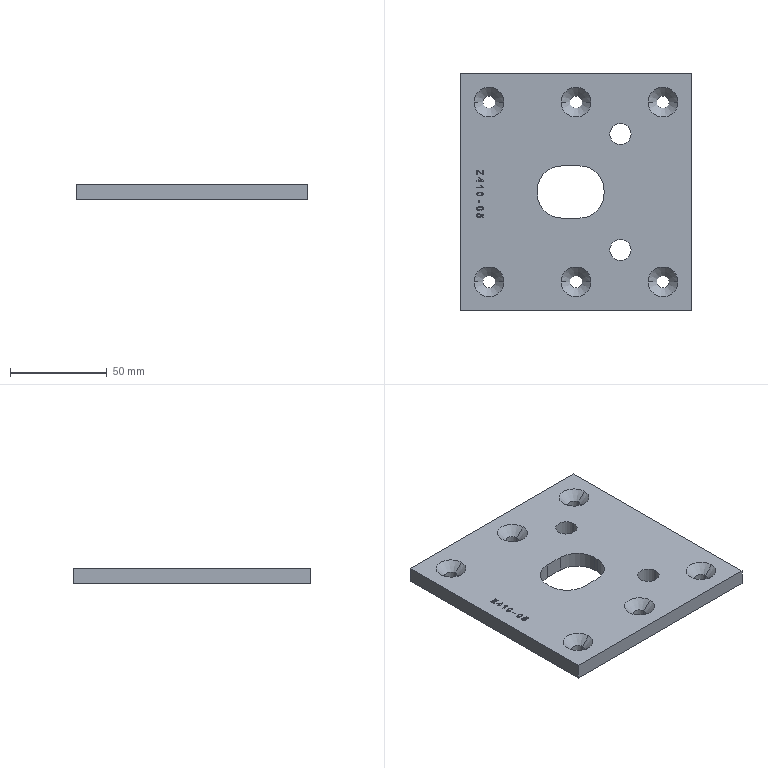Part | Creo | 1 solid | 153 faces | box 120 x 123 x 8 mm | volume 106820 mm3 | other 67 | plane 53 | cylinder 21 | cone 12 | commonest cylinder face diameters 6.4 x12 11 x4 25 x4 45.582 x1